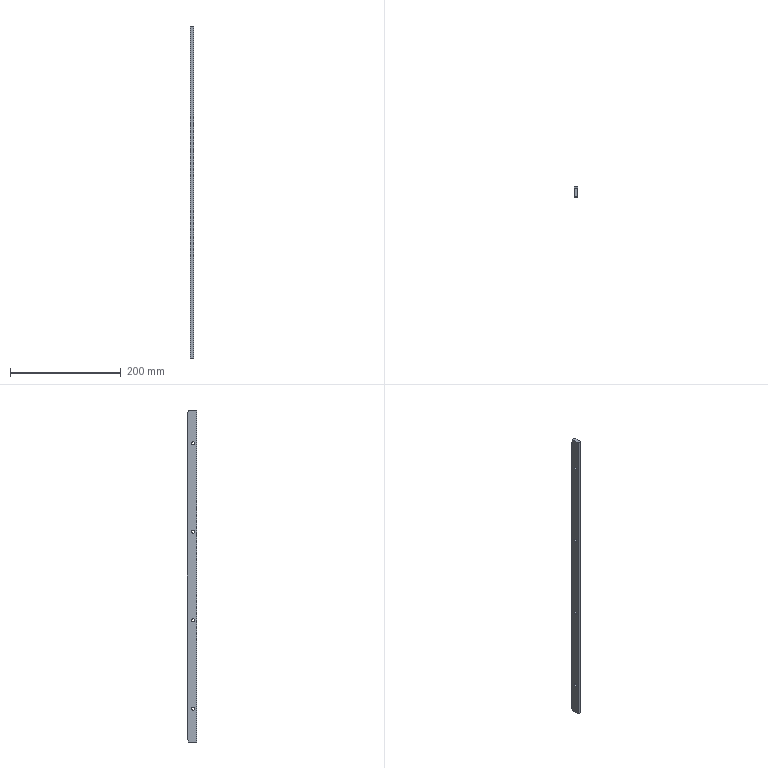Part | STEP file | 0228_206_Guide | 1 solid | 16 faces | box 6 x 18 x 600 mm | volume 64069 mm3 | cylinder 8 | plane 8 | commonest cylinder face diameters 5.5 x8
STEP:
#1=CARTESIAN_POINT('',(0.,0.,0.));
#2=DIRECTION('',(0.,0.,1.));
#3=DIRECTION('',(1.,0.,0.));
#4=AXIS2_PLACEMENT_3D('',#1,#2,#3);
#5=CARTESIAN_POINT('',(-6.,7.,237.25));
#6=VERTEX_POINT('',#5);
#7=CARTESIAN_POINT('',(0.,7.,237.25));
#8=VERTEX_POINT('',#7);
#9=CARTESIAN_POINT('',(0.,7.,237.25));
#10=DIRECTION('',(1.,0.,0.));
#11=VECTOR('',#10,1.);
#12=LINE('',#9,#11);
#13=CARTESIAN_POINT('',(0.,7.,240.));
#14=DIRECTION('',(1.,0.,0.));
#15=DIRECTION('',(0.,0.,-1.));
#16=AXIS2_PLACEMENT_3D('',#13,#14,#15);
#17=CYLINDRICAL_SURFACE('',#16,2.75);
#18=CARTESIAN_POINT('',(6.283,0.));
#19=DIRECTION('',(0.,1.));
#20=VECTOR('',#19,1.);
#21=LINE('',#18,#20);
#22=(GEOMETRIC_REPRESENTATION_CONTEXT(2)PARAMETRIC_REPRESENTATION_CONTEXT()REPRESENTATION_CONTEXT('',''));
#23=DEFINITIONAL_REPRESENTATION('',(#21),#22);
#24=PCURVE('',#17,#23);
#25=CARTESIAN_POINT('',(0.,7.,240.));
#26=DIRECTION('',(1.,0.,0.));
#27=DIRECTION('',(0.,0.,-1.));
#28=AXIS2_PLACEMENT_3D('',#25,#26,#27);
#29=CYLINDRICAL_SURFACE('',#28,2.75);
#30=CARTESIAN_POINT('',(0.,0.));
#31=DIRECTION('',(0.,1.));
#32=VECTOR('',#31,1.);
#33=LINE('',#30,#32);
#34=(GEOMETRIC_REPRESENTATION_CONTEXT(2)PARAMETRIC_REPRESENTATION_CONTEXT()REPRESENTATION_CONTEXT('',''));
#35=DEFINITIONAL_REPRESENTATION('',(#33),#34);
#36=PCURVE('',#29,#35);
#37=SURFACE_CURVE('',#12,(#24,#36),.PCURVE_S1.);
#38=EDGE_CURVE('',#6,#8,#37,.T.);
#39=ORIENTED_EDGE('',*,*,#38,.T.);
#40=CARTESIAN_POINT('',(0.,7.,242.75));
#41=VERTEX_POINT('',#40);
#42=CARTESIAN_POINT('',(0.,7.,240.));
#43=DIRECTION('',(1.,0.,0.));
#44=DIRECTION('',(0.,0.,-1.));
#45=AXIS2_PLACEMENT_3D('',#42,#43,#44);
#46=CIRCLE('',#45,2.75);
#47=CARTESIAN_POINT('',(0.,0.));
#48=DIRECTION('',(1.,0.));
#49=VECTOR('',#48,1.);
#50=LINE('',#47,#49);
#51=(GEOMETRIC_REPRESENTATION_CONTEXT(2)PARAMETRIC_REPRESENTATION_CONTEXT()REPRESENTATION_CONTEXT('',''));
#52=DEFINITIONAL_REPRESENTATION('',(#50),#51);
#53=PCURVE('',#17,#52);
#54=CARTESIAN_POINT('',(0.,18.,-300.));
#55=DIRECTION('',(1.,0.,0.));
#56=DIRECTION('',(0.,0.,-1.));
#57=AXIS2_PLACEMENT_3D('',#54,#55,#56);
#58=PLANE('',#57);
#59=CARTESIAN_POINT('',(-540.,-11.));
#60=DIRECTION('',(1.,0.));
#61=AXIS2_PLACEMENT_2D('',#59,#60);
#62=CIRCLE('',#61,2.75);
#63=(GEOMETRIC_REPRESENTATION_CONTEXT(2)PARAMETRIC_REPRESENTATION_CONTEXT()REPRESENTATION_CONTEXT('',''));
#64=DEFINITIONAL_REPRESENTATION('',(#62),#63);
#65=PCURVE('',#58,#64);
#66=SURFACE_CURVE('',#46,(#53,#65),.PCURVE_S1.);
#67=EDGE_CURVE('',#41,#8,#66,.T.);
#68=ORIENTED_EDGE('',*,*,#67,.F.);
#69=CARTESIAN_POINT('',(-6.,7.,242.75));
#70=VERTEX_POINT('',#69);
#71=CARTESIAN_POINT('',(0.,7.,242.75));
#72=DIRECTION('',(1.,0.,0.));
#73=VECTOR('',#72,1.);
#74=LINE('',#71,#73);
#75=CARTESIAN_POINT('',(3.142,0.));
#76=DIRECTION('',(0.,1.));
#77=VECTOR('',#76,1.);
#78=LINE('',#75,#77);
#79=(GEOMETRIC_REPRESENTATION_CONTEXT(2)PARAMETRIC_REPRESENTATION_CONTEXT()REPRESENTATION_CONTEXT('',''));
#80=DEFINITIONAL_REPRESENTATION('',(#78),#79);
#81=PCURVE('',#17,#80);
#82=CARTESIAN_POINT('',(3.142,0.));
#83=DIRECTION('',(0.,1.));
#84=VECTOR('',#83,1.);
#85=LINE('',#82,#84);
#86=(GEOMETRIC_REPRESENTATION_CONTEXT(2)PARAMETRIC_REPRESENTATION_CONTEXT()REPRESENTATION_CONTEXT('',''));
#87=DEFINITIONAL_REPRESENTATION('',(#85),#86);
#88=PCURVE('',#29,#87);
#89=SURFACE_CURVE('',#74,(#81,#88),.PCURVE_S1.);
#90=EDGE_CURVE('',#70,#41,#89,.T.);
#91=ORIENTED_EDGE('',*,*,#90,.F.);
#92=CARTESIAN_POINT('',(-6.,7.,240.));
#93=DIRECTION('',(1.,0.,0.));
#94=DIRECTION('',(0.,0.,-1.));
#95=AXIS2_PLACEMENT_3D('',#92,#93,#94);
#96=CIRCLE('',#95,2.75);
#97=CARTESIAN_POINT('',(0.,-6.));
#98=DIRECTION('',(1.,0.));
#99=VECTOR('',#98,1.);
#100=LINE('',#97,#99);
#101=(GEOMETRIC_REPRESENTATION_CONTEXT(2)PARAMETRIC_REPRESENTATION_CONTEXT()REPRESENTATION_CONTEXT('',''));
#102=DEFINITIONAL_REPRESENTATION('',(#100),#101);
#103=PCURVE('',#17,#102);
#104=CARTESIAN_POINT('',(-6.,18.,-300.));
#105=DIRECTION('',(1.,0.,0.));
#106=DIRECTION('',(0.,0.,-1.));
#107=AXIS2_PLACEMENT_3D('',#104,#105,#106);
#108=PLANE('',#107);
#109=CARTESIAN_POINT('',(-540.,-11.));
#110=DIRECTION('',(1.,0.));
#111=AXIS2_PLACEMENT_2D('',#109,#110);
#112=CIRCLE('',#111,2.75);
#113=(GEOMETRIC_REPRESENTATION_CONTEXT(2)PARAMETRIC_REPRESENTATION_CONTEXT()REPRESENTATION_CONTEXT('',''));
#114=DEFINITIONAL_REPRESENTATION('',(#112),#113);
#115=PCURVE('',#108,#114);
#116=SURFACE_CURVE('',#96,(#103,#115),.PCURVE_S1.);
#117=EDGE_CURVE('',#70,#6,#116,.T.);
#118=ORIENTED_EDGE('',*,*,#117,.T.);
#119=EDGE_LOOP('',(#39,#68,#91,#118));
#120=FACE_BOUND('',#119,.F.);
#121=ADVANCED_FACE('',(#120),#17,.F.);
#122=CARTESIAN_POINT('',(-6.,7.,77.25));
#123=VERTEX_POINT('',#122);
#124=CARTESIAN_POINT('',(0.,7.,77.25));
#125=VERTEX_POINT('',#124);
#126=CARTESIAN_POINT('',(0.,7.,77.25));
#127=DIRECTION('',(1.,0.,0.));
#128=VECTOR('',#127,1.);
#129=LINE('',#126,#128);
#130=CARTESIAN_POINT('',(0.,7.,80.));
#131=DIRECTION('',(1.,0.,0.));
#132=DIRECTION('',(0.,0.,-1.));
#133=AXIS2_PLACEMENT_3D('',#130,#131,#132);
#134=CYLINDRICAL_SURFACE('',#133,2.75);
#135=CARTESIAN_POINT('',(6.283,0.));
#136=DIRECTION('',(0.,1.));
#137=VECTOR('',#136,1.);
#138=LINE('',#135,#137);
#139=(GEOMETRIC_REPRESENTATION_CONTEXT(2)PARAMETRIC_REPRESENTATION_CONTEXT()REPRESENTATION_CONTEXT('',''));
#140=DEFINITIONAL_REPRESENTATION('',(#138),#139);
#141=PCURVE('',#134,#140);
#142=CARTESIAN_POINT('',(0.,7.,80.));
#143=DIRECTION('',(1.,0.,0.));
#144=DIRECTION('',(0.,0.,-1.));
#145=AXIS2_PLACEMENT_3D('',#142,#143,#144);
#146=CYLINDRICAL_SURFACE('',#145,2.75);
#147=CARTESIAN_POINT('',(0.,0.));
#148=DIRECTION('',(0.,1.));
#149=VECTOR('',#148,1.);
#150=LINE('',#147,#149);
#151=(GEOMETRIC_REPRESENTATION_CONTEXT(2)PARAMETRIC_REPRESENTATION_CONTEXT()REPRESENTATION_CONTEXT('',''));
#152=DEFINITIONAL_REPRESENTATION('',(#150),#151);
#153=PCURVE('',#146,#152);
#154=SURFACE_CURVE('',#129,(#141,#153),.PCURVE_S1.);
#155=EDGE_CURVE('',#123,#125,#154,.T.);
#156=ORIENTED_EDGE('',*,*,#155,.T.);
#157=CARTESIAN_POINT('',(0.,7.,82.75));
#158=VERTEX_POINT('',#157);
#159=CARTESIAN_POINT('',(0.,7.,80.));
#160=DIRECTION('',(1.,0.,0.));
#161=DIRECTION('',(0.,0.,-1.));
#162=AXIS2_PLACEMENT_3D('',#159,#160,#161);
#163=CIRCLE('',#162,2.75);
#164=CARTESIAN_POINT('',(0.,0.));
#165=DIRECTION('',(1.,0.));
#166=VECTOR('',#165,1.);
#167=LINE('',#164,#166);
#168=(GEOMETRIC_REPRESENTATION_CONTEXT(2)PARAMETRIC_REPRESENTATION_CONTEXT()REPRESENTATION_CONTEXT('',''));
#169=DEFINITIONAL_REPRESENTATION('',(#167),#168);
#170=PCURVE('',#134,#169);
#171=CARTESIAN_POINT('',(-380.,-11.));
#172=DIRECTION('',(1.,0.));
#173=AXIS2_PLACEMENT_2D('',#171,#172);
#174=CIRCLE('',#173,2.75);
#175=(GEOMETRIC_REPRESENTATION_CONTEXT(2)PARAMETRIC_REPRESENTATION_CONTEXT()REPRESENTATION_CONTEXT('',''));
#176=DEFINITIONAL_REPRESENTATION('',(#174),#175);
#177=PCURVE('',#58,#176);
#178=SURFACE_CURVE('',#163,(#170,#177),.PCURVE_S1.);
#179=EDGE_CURVE('',#158,#125,#178,.T.);
#180=ORIENTED_EDGE('',*,*,#179,.F.);
#181=CARTESIAN_POINT('',(-6.,7.,82.75));
#182=VERTEX_POINT('',#181);
#183=CARTESIAN_POINT('',(0.,7.,82.75));
#184=DIRECTION('',(1.,0.,0.));
#185=VECTOR('',#184,1.);
#186=LINE('',#183,#185);
#187=CARTESIAN_POINT('',(3.142,0.));
#188=DIRECTION('',(0.,1.));
#189=VECTOR('',#188,1.);
#190=LINE('',#187,#189);
#191=(GEOMETRIC_REPRESENTATION_CONTEXT(2)PARAMETRIC_REPRESENTATION_CONTEXT()REPRESENTATION_CONTEXT('',''));
#192=DEFINITIONAL_REPRESENTATION('',(#190),#191);
#193=PCURVE('',#134,#192);
#194=CARTESIAN_POINT('',(3.142,0.));
#195=DIRECTION('',(0.,1.));
#196=VECTOR('',#195,1.);
#197=LINE('',#194,#196);
#198=(GEOMETRIC_REPRESENTATION_CONTEXT(2)PARAMETRIC_REPRESENTATION_CONTEXT()REPRESENTATION_CONTEXT('',''));
#199=DEFINITIONAL_REPRESENTATION('',(#197),#198);
#200=PCURVE('',#146,#199);
#201=SURFACE_CURVE('',#186,(#193,#200),.PCURVE_S1.);
#202=EDGE_CURVE('',#182,#158,#201,.T.);
#203=ORIENTED_EDGE('',*,*,#202,.F.);
#204=CARTESIAN_POINT('',(-6.,7.,80.));
#205=DIRECTION('',(1.,0.,0.));
#206=DIRECTION('',(0.,0.,-1.));
#207=AXIS2_PLACEMENT_3D('',#204,#205,#206);
#208=CIRCLE('',#207,2.75);
#209=CARTESIAN_POINT('',(0.,-6.));
#210=DIRECTION('',(1.,0.));
#211=VECTOR('',#210,1.);
#212=LINE('',#209,#211);
#213=(GEOMETRIC_REPRESENTATION_CONTEXT(2)PARAMETRIC_REPRESENTATION_CONTEXT()REPRESENTATION_CONTEXT('',''));
#214=DEFINITIONAL_REPRESENTATION('',(#212),#213);
#215=PCURVE('',#134,#214);
#216=CARTESIAN_POINT('',(-380.,-11.));
#217=DIRECTION('',(1.,0.));
#218=AXIS2_PLACEMENT_2D('',#216,#217);
#219=CIRCLE('',#218,2.75);
#220=(GEOMETRIC_REPRESENTATION_CONTEXT(2)PARAMETRIC_REPRESENTATION_CONTEXT()REPRESENTATION_CONTEXT('',''));
#221=DEFINITIONAL_REPRESENTATION('',(#219),#220);
#222=PCURVE('',#108,#221);
#223=SURFACE_CURVE('',#208,(#215,#222),.PCURVE_S1.);
#224=EDGE_CURVE('',#182,#123,#223,.T.);
#225=ORIENTED_EDGE('',*,*,#224,.T.);
#226=EDGE_LOOP('',(#156,#180,#203,#225));
#227=FACE_BOUND('',#226,.F.);
#228=ADVANCED_FACE('',(#227),#134,.F.);
#229=CARTESIAN_POINT('',(-6.,7.,-82.75));
#230=VERTEX_POINT('',#229);
#231=CARTESIAN_POINT('',(0.,7.,-82.75));
#232=VERTEX_POINT('',#231);
#233=CARTESIAN_POINT('',(0.,7.,-82.75));
#234=DIRECTION('',(1.,0.,0.));
#235=VECTOR('',#234,1.);
#236=LINE('',#233,#235);
#237=CARTESIAN_POINT('',(0.,7.,-80.));
#238=DIRECTION('',(1.,0.,0.));
#239=DIRECTION('',(0.,0.,-1.));
#240=AXIS2_PLACEMENT_3D('',#237,#238,#239);
#241=CYLINDRICAL_SURFACE('',#240,2.75);
#242=CARTESIAN_POINT('',(6.283,0.));
#243=DIRECTION('',(0.,1.));
#244=VECTOR('',#243,1.);
#245=LINE('',#242,#244);
#246=(GEOMETRIC_REPRESENTATION_CONTEXT(2)PARAMETRIC_REPRESENTATION_CONTEXT()REPRESENTATION_CONTEXT('',''));
#247=DEFINITIONAL_REPRESENTATION('',(#245),#246);
#248=PCURVE('',#241,#247);
#249=CARTESIAN_POINT('',(0.,7.,-80.));
#250=DIRECTION('',(1.,0.,0.));
#251=DIRECTION('',(0.,0.,-1.));
#252=AXIS2_PLACEMENT_3D('',#249,#250,#251);
#253=CYLINDRICAL_SURFACE('',#252,2.75);
#254=CARTESIAN_POINT('',(0.,0.));
#255=DIRECTION('',(0.,1.));
#256=VECTOR('',#255,1.);
#257=LINE('',#254,#256);
#258=(GEOMETRIC_REPRESENTATION_CONTEXT(2)PARAMETRIC_REPRESENTATION_CONTEXT()REPRESENTATION_CONTEXT('',''));
#259=DEFINITIONAL_REPRESENTATION('',(#257),#258);
#260=PCURVE('',#253,#259);
#261=SURFACE_CURVE('',#236,(#248,#260),.PCURVE_S1.);
#262=EDGE_CURVE('',#230,#232,#261,.T.);
#263=ORIENTED_EDGE('',*,*,#262,.T.);
#264=CARTESIAN_POINT('',(0.,7.,-77.25));
#265=VERTEX_POINT('',#264);
#266=CARTESIAN_POINT('',(0.,7.,-80.));
#267=DIRECTION('',(1.,0.,0.));
#268=DIRECTION('',(0.,0.,-1.));
#269=AXIS2_PLACEMENT_3D('',#266,#267,#268);
#270=CIRCLE('',#269,2.75);
#271=CARTESIAN_POINT('',(0.,0.));
#272=DIRECTION('',(1.,0.));
#273=VECTOR('',#272,1.);
#274=LINE('',#271,#273);
#275=(GEOMETRIC_REPRESENTATION_CONTEXT(2)PARAMETRIC_REPRESENTATION_CONTEXT()REPRESENTATION_CONTEXT('',''));
#276=DEFINITIONAL_REPRESENTATION('',(#274),#275);
#277=PCURVE('',#241,#276);
#278=CARTESIAN_POINT('',(-220.,-11.));
#279=DIRECTION('',(1.,0.));
#280=AXIS2_PLACEMENT_2D('',#278,#279);
#281=CIRCLE('',#280,2.75);
#282=(GEOMETRIC_REPRESENTATION_CONTEXT(2)PARAMETRIC_REPRESENTATION_CONTEXT()REPRESENTATION_CONTEXT('',''));
#283=DEFINITIONAL_REPRESENTATION('',(#281),#282);
#284=PCURVE('',#58,#283);
#285=SURFACE_CURVE('',#270,(#277,#284),.PCURVE_S1.);
#286=EDGE_CURVE('',#265,#232,#285,.T.);
#287=ORIENTED_EDGE('',*,*,#286,.F.);
#288=CARTESIAN_POINT('',(-6.,7.,-77.25));
#289=VERTEX_POINT('',#288);
#290=CARTESIAN_POINT('',(0.,7.,-77.25));
#291=DIRECTION('',(1.,0.,0.));
#292=VECTOR('',#291,1.);
#293=LINE('',#290,#292);
#294=CARTESIAN_POINT('',(3.142,0.));
#295=DIRECTION('',(0.,1.));
#296=VECTOR('',#295,1.);
#297=LINE('',#294,#296);
#298=(GEOMETRIC_REPRESENTATION_CONTEXT(2)PARAMETRIC_REPRESENTATION_CONTEXT()REPRESENTATION_CONTEXT('',''));
#299=DEFINITIONAL_REPRESENTATION('',(#297),#298);
#300=PCURVE('',#241,#299);
#301=CARTESIAN_POINT('',(3.142,0.));
#302=DIRECTION('',(0.,1.));
#303=VECTOR('',#302,1.);
#304=LINE('',#301,#303);
#305=(GEOMETRIC_REPRESENTATION_CONTEXT(2)PARAMETRIC_REPRESENTATION_CONTEXT()REPRESENTATION_CONTEXT('',''));
#306=DEFINITIONAL_REPRESENTATION('',(#304),#305);
#307=PCURVE('',#253,#306);
#308=SURFACE_CURVE('',#293,(#300,#307),.PCURVE_S1.);
#309=EDGE_CURVE('',#289,#265,#308,.T.);
#310=ORIENTED_EDGE('',*,*,#309,.F.);
#311=CARTESIAN_POINT('',(-6.,7.,-80.));
#312=DIRECTION('',(1.,0.,0.));
#313=DIRECTION('',(0.,0.,-1.));
#314=AXIS2_PLACEMENT_3D('',#311,#312,#313);
#315=CIRCLE('',#314,2.75);
#316=CARTESIAN_POINT('',(0.,-6.));
#317=DIRECTION('',(1.,0.));
#318=VECTOR('',#317,1.);
#319=LINE('',#316,#318);
#320=(GEOMETRIC_REPRESENTATION_CONTEXT(2)PARAMETRIC_REPRESENTATION_CONTEXT()REPRESENTATION_CONTEXT('',''));
#321=DEFINITIONAL_REPRESENTATION('',(#319),#320);
#322=PCURVE('',#241,#321);
#323=CARTESIAN_POINT('',(-220.,-11.));
#324=DIRECTION('',(1.,0.));
#325=AXIS2_PLACEMENT_2D('',#323,#324);
#326=CIRCLE('',#325,2.75);
#327=(GEOMETRIC_REPRESENTATION_CONTEXT(2)PARAMETRIC_REPRESENTATION_CONTEXT()REPRESENTATION_CONTEXT('',''));
#328=DEFINITIONAL_REPRESENTATION('',(#326),#327);
#329=PCURVE('',#108,#328);
#330=SURFACE_CURVE('',#315,(#322,#329),.PCURVE_S1.);
#331=EDGE_CURVE('',#289,#230,#330,.T.);
#332=ORIENTED_EDGE('',*,*,#331,.T.);
#333=EDGE_LOOP('',(#263,#287,#310,#332));
#334=FACE_BOUND('',#333,.F.);
#335=ADVANCED_FACE('',(#334),#241,.F.);
#336=CARTESIAN_POINT('',(-6.,7.,-242.75));
#337=VERTEX_POINT('',#336);
#338=CARTESIAN_POINT('',(0.,7.,-242.75));
#339=VERTEX_POINT('',#338);
#340=CARTESIAN_POINT('',(0.,7.,-242.75));
#341=DIRECTION('',(1.,0.,0.));
#342=VECTOR('',#341,1.);
#343=LINE('',#340,#342);
#344=CARTESIAN_POINT('',(0.,7.,-240.));
#345=DIRECTION('',(1.,0.,0.));
#346=DIRECTION('',(0.,0.,-1.));
#347=AXIS2_PLACEMENT_3D('',#344,#345,#346);
#348=CYLINDRICAL_SURFACE('',#347,2.75);
#349=CARTESIAN_POINT('',(6.283,0.));
#350=DIRECTION('',(0.,1.));
#351=VECTOR('',#350,1.);
#352=LINE('',#349,#351);
#353=(GEOMETRIC_REPRESENTATION_CONTEXT(2)PARAMETRIC_REPRESENTATION_CONTEXT()REPRESENTATION_CONTEXT('',''));
#354=DEFINITIONAL_REPRESENTATION('',(#352),#353);
#355=PCURVE('',#348,#354);
#356=CARTESIAN_POINT('',(0.,7.,-240.));
#357=DIRECTION('',(1.,0.,0.));
#358=DIRECTION('',(0.,0.,-1.));
#359=AXIS2_PLACEMENT_3D('',#356,#357,#358);
#360=CYLINDRICAL_SURFACE('',#359,2.75);
#361=CARTESIAN_POINT('',(0.,0.));
#362=DIRECTION('',(0.,1.));
#363=VECTOR('',#362,1.);
#364=LINE('',#361,#363);
#365=(GEOMETRIC_REPRESENTATION_CONTEXT(2)PARAMETRIC_REPRESENTATION_CONTEXT()REPRESENTATION_CONTEXT('',''));
#366=DEFINITIONAL_REPRESENTATION('',(#364),#365);
#367=PCURVE('',#360,#366);
#368=SURFACE_CURVE('',#343,(#355,#367),.PCURVE_S1.);
#369=EDGE_CURVE('',#337,#339,#368,.T.);
#370=ORIENTED_EDGE('',*,*,#369,.T.);
#371=CARTESIAN_POINT('',(0.,7.,-237.25));
#372=VERTEX_POINT('',#371);
#373=CARTESIAN_POINT('',(0.,7.,-240.));
#374=DIRECTION('',(1.,0.,0.));
#375=DIRECTION('',(0.,0.,-1.));
#376=AXIS2_PLACEMENT_3D('',#373,#374,#375);
#377=CIRCLE('',#376,2.75);
#378=CARTESIAN_POINT('',(0.,0.));
#379=DIRECTION('',(1.,0.));
#380=VECTOR('',#379,1.);
#381=LINE('',#378,#380);
#382=(GEOMETRIC_REPRESENTATION_CONTEXT(2)PARAMETRIC_REPRESENTATION_CONTEXT()REPRESENTATION_CONTEXT('',''));
#383=DEFINITIONAL_REPRESENTATION('',(#381),#382);
#384=PCURVE('',#348,#383);
#385=CARTESIAN_POINT('',(-60.,-11.));
#386=DIRECTION('',(1.,0.));
#387=AXIS2_PLACEMENT_2D('',#385,#386);
#388=CIRCLE('',#387,2.75);
#389=(GEOMETRIC_REPRESENTATION_CONTEXT(2)PARAMETRIC_REPRESENTATION_CONTEXT()REPRESENTATION_CONTEXT('',''));
#390=DEFINITIONAL_REPRESENTATION('',(#388),#389);
#391=PCURVE('',#58,#390);
#392=SURFACE_CURVE('',#377,(#384,#391),.PCURVE_S1.);
#393=EDGE_CURVE('',#372,#339,#392,.T.);
#394=ORIENTED_EDGE('',*,*,#393,.F.);
#395=CARTESIAN_POINT('',(-6.,7.,-237.25));
#396=VERTEX_POINT('',#395);
#397=CARTESIAN_POINT('',(0.,7.,-237.25));
#398=DIRECTION('',(1.,0.,0.));
#399=VECTOR('',#398,1.);
#400=LINE('',#397,#399);
#401=CARTESIAN_POINT('',(3.142,0.));
#402=DIRECTION('',(0.,1.));
#403=VECTOR('',#402,1.);
#404=LINE('',#401,#403);
#405=(GEOMETRIC_REPRESENTATION_CONTEXT(2)PARAMETRIC_REPRESENTATION_CONTEXT()REPRESENTATION_CONTEXT('',''));
#406=DEFINITIONAL_REPRESENTATION('',(#404),#405);
#407=PCURVE('',#348,#406);
#408=CARTESIAN_POINT('',(3.142,0.));
#409=DIRECTION('',(0.,1.));
#410=VECTOR('',#409,1.);
#411=LINE('',#408,#410);
#412=(GEOMETRIC_REPRESENTATION_CONTEXT(2)PARAMETRIC_REPRESENTATION_CONTEXT()REPRESENTATION_CONTEXT('',''));
#413=DEFINITIONAL_REPRESENTATION('',(#411),#412);
#414=PCURVE('',#360,#413);
#415=SURFACE_CURVE('',#400,(#407,#414),.PCURVE_S1.);
#416=EDGE_CURVE('',#396,#372,#415,.T.);
#417=ORIENTED_EDGE('',*,*,#416,.F.);
#418=CARTESIAN_POINT('',(-6.,7.,-240.));
#419=DIRECTION('',(1.,0.,0.));
#420=DIRECTION('',(0.,0.,-1.));
#421=AXIS2_PLACEMENT_3D('',#418,#419,#420);
#422=CIRCLE('',#421,2.75);
#423=CARTESIAN_POINT('',(0.,-6.));
#424=DIRECTION('',(1.,0.));
#425=VECTOR('',#424,1.);
#426=LINE('',#423,#425);
#427=(GEOMETRIC_REPRESENTATION_CONTEXT(2)PARAMETRIC_REPRESENTATION_CONTEXT()REPRESENTATION_CONTEXT('',''));
#428=DEFINITIONAL_REPRESENTATION('',(#426),#427);
#429=PCURVE('',#348,#428);
#430=CARTESIAN_POINT('',(-60.,-11.));
#431=DIRECTION('',(1.,0.));
#432=AXIS2_PLACEMENT_2D('',#430,#431);
#433=CIRCLE('',#432,2.75);
#434=(GEOMETRIC_REPRESENTATION_CONTEXT(2)PARAMETRIC_REPRESENTATION_CONTEXT()REPRESENTATION_CONTEXT('',''));
#435=DEFINITIONAL_REPRESENTATION('',(#433),#434);
#436=PCURVE('',#108,#435);
#437=SURFACE_CURVE('',#422,(#429,#436),.PCURVE_S1.);
#438=EDGE_CURVE('',#396,#337,#437,.T.);
#439=ORIENTED_EDGE('',*,*,#438,.T.);
#440=EDGE_LOOP('',(#370,#394,#417,#439));
#441=FACE_BOUND('',#440,.F.);
#442=ADVANCED_FACE('',(#441),#348,.F.);
#443=CARTESIAN_POINT('',(-6.,0.,-300.));
#444=VERTEX_POINT('',#443);
#445=CARTESIAN_POINT('',(-6.,15.321,-300.));
#446=VERTEX_POINT('',#445);
#447=CARTESIAN_POINT('',(-6.,0.,-300.));
#448=DIRECTION('',(0.,1.,0.));
#449=VECTOR('',#448,1.);
#450=LINE('',#447,#449);
#451=CARTESIAN_POINT('',(-6.,0.,-300.));
#452=DIRECTION('',(0.,0.,-1.));
#453=DIRECTION('',(-1.,0.,0.));
#454=AXIS2_PLACEMENT_3D('',#451,#452,#453);
#455=PLANE('',#454);
#456=CARTESIAN_POINT('',(0.,0.));
#457=DIRECTION('',(0.,1.));
#458=VECTOR('',#457,1.);
#459=LINE('',#456,#458);
#460=(GEOMETRIC_REPRESENTATION_CONTEXT(2)PARAMETRIC_REPRESENTATION_CONTEXT()REPRESENTATION_CONTEXT('',''));
#461=DEFINITIONAL_REPRESENTATION('',(#459),#460);
#462=PCURVE('',#455,#461);
#463=CARTESIAN_POINT('',(0.,-18.));
#464=DIRECTION('',(0.,1.));
#465=VECTOR('',#464,1.);
#466=LINE('',#463,#465);
#467=(GEOMETRIC_REPRESENTATION_CONTEXT(2)PARAMETRIC_REPRESENTATION_CONTEXT()REPRESENTATION_CONTEXT('',''));
#468=DEFINITIONAL_REPRESENTATION('',(#466),#467);
#469=PCURVE('',#108,#468);
#470=SURFACE_CURVE('',#450,(#462,#469),.PCURVE_S1.);
#471=EDGE_CURVE('',#444,#446,#470,.T.);
#472=ORIENTED_EDGE('',*,*,#471,.T.);
#473=CARTESIAN_POINT('',(0.,15.321,-300.));
#474=VERTEX_POINT('',#473);
#475=CARTESIAN_POINT('',(-6.,15.321,-300.));
#476=DIRECTION('',(1.,0.,0.));
#477=VECTOR('',#476,1.);
#478=LINE('',#475,#477);
#479=CARTESIAN_POINT('',(0.,15.321));
#480=DIRECTION('',(-1.,0.));
#481=VECTOR('',#480,1.);
#482=LINE('',#479,#481);
#483=(GEOMETRIC_REPRESENTATION_CONTEXT(2)PARAMETRIC_REPRESENTATION_CONTEXT()REPRESENTATION_CONTEXT('',''));
#484=DEFINITIONAL_REPRESENTATION('',(#482),#483);
#485=PCURVE('',#455,#484);
#486=CARTESIAN_POINT('',(-6.,15.321,-300.));
#487=DIRECTION('',(0.,-0.9659,0.2588));
#488=DIRECTION('',(0.,-0.2588,-0.9659));
#489=AXIS2_PLACEMENT_3D('',#486,#487,#488);
#490=PLANE('',#489);
#491=CARTESIAN_POINT('',(0.,0.));
#492=DIRECTION('',(0.,1.));
#493=VECTOR('',#492,1.);
#494=LINE('',#491,#493);
#495=(GEOMETRIC_REPRESENTATION_CONTEXT(2)PARAMETRIC_REPRESENTATION_CONTEXT()REPRESENTATION_CONTEXT('',''));
#496=DEFINITIONAL_REPRESENTATION('',(#494),#495);
#497=PCURVE('',#490,#496);
#498=SURFACE_CURVE('',#478,(#485,#497),.PCURVE_S1.);
#499=EDGE_CURVE('',#446,#474,#498,.T.);
#500=ORIENTED_EDGE('',*,*,#499,.T.);
#501=CARTESIAN_POINT('',(0.,0.,-300.));
#502=VERTEX_POINT('',#501);
#503=CARTESIAN_POINT('',(0.,0.,-300.));
#504=DIRECTION('',(0.,1.,0.));
#505=VECTOR('',#504,1.);
#506=LINE('',#503,#505);
#507=CARTESIAN_POINT('',(-6.,0.));
#508=DIRECTION('',(0.,1.));
#509=VECTOR('',#508,1.);
#510=LINE('',#507,#509);
#511=(GEOMETRIC_REPRESENTATION_CONTEXT(2)PARAMETRIC_REPRESENTATION_CONTEXT()REPRESENTATION_CONTEXT('',''));
#512=DEFINITIONAL_REPRESENTATION('',(#510),#511);
#513=PCURVE('',#455,#512);
#514=CARTESIAN_POINT('',(0.,-18.));
#515=DIRECTION('',(0.,1.));
#516=VECTOR('',#515,1.);
#517=LINE('',#514,#516);
#518=(GEOMETRIC_REPRESENTATION_CONTEXT(2)PARAMETRIC_REPRESENTATION_CONTEXT()REPRESENTATION_CONTEXT('',''));
#519=DEFINITIONAL_REPRESENTATION('',(#517),#518);
#520=PCURVE('',#58,#519);
#521=SURFACE_CURVE('',#506,(#513,#520),.PCURVE_S1.);
#522=EDGE_CURVE('',#502,#474,#521,.T.);
#523=ORIENTED_EDGE('',*,*,#522,.F.);
#524=CARTESIAN_POINT('',(-6.,0.,-300.));
#525=DIRECTION('',(1.,0.,0.));
#526=VECTOR('',#525,1.);
#527=LINE('',#524,#526);
#528=CARTESIAN_POINT('',(0.,0.));
#529=DIRECTION('',(-1.,0.));
#530=VECTOR('',#529,1.);
#531=LINE('',#528,#530);
#532=(GEOMETRIC_REPRESENTATION_CONTEXT(2)PARAMETRIC_REPRESENTATION_CONTEXT()REPRESENTATION_CONTEXT('',''));
#533=DEFINITIONAL_REPRESENTATION('',(#531),#532);
#534=PCURVE('',#455,#533);
#535=CARTESIAN_POINT('',(-6.,0.,-300.));
#536=DIRECTION('',(0.,-1.,0.));
#537=DIRECTION('',(0.,0.,-1.));
#538=AXIS2_PLACEMENT_3D('',#535,#536,#537);
#539=PLANE('',#538);
#540=CARTESIAN_POINT('',(0.,0.));
#541=DIRECTION('',(0.,1.));
#542=VECTOR('',#541,1.);
#543=LINE('',#540,#542);
#544=(GEOMETRIC_REPRESENTATION_CONTEXT(2)PARAMETRIC_REPRESENTATION_CONTEXT()REPRESENTATION_CONTEXT('',''));
#545=DEFINITIONAL_REPRESENTATION('',(#543),#544);
#546=PCURVE('',#539,#545);
#547=SURFACE_CURVE('',#527,(#534,#546),.PCURVE_S1.);
#548=EDGE_CURVE('',#444,#502,#547,.T.);
#549=ORIENTED_EDGE('',*,*,#548,.F.);
#550=EDGE_LOOP('',(#472,#500,#523,#549));
#551=FACE_BOUND('',#550,.T.);
#552=ADVANCED_FACE('',(#551),#455,.T.);
#553=CARTESIAN_POINT('',(0.,0.,300.));
#554=VERTEX_POINT('',#553);
#555=CARTESIAN_POINT('',(0.,0.,-300.));
#556=DIRECTION('',(0.,0.,-1.));
#557=VECTOR('',#556,1.);
#558=LINE('',#555,#557);
#559=CARTESIAN_POINT('',(0.,6.));
#560=DIRECTION('',(1.,0.));
#561=VECTOR('',#560,1.);
#562=LINE('',#559,#561);
#563=(GEOMETRIC_REPRESENTATION_CONTEXT(2)PARAMETRIC_REPRESENTATION_CONTEXT()REPRESENTATION_CONTEXT('',''));
#564=DEFINITIONAL_REPRESENTATION('',(#562),#563);
#565=PCURVE('',#539,#564);
#566=CARTESIAN_POINT('',(0.,-18.));
#567=DIRECTION('',(1.,0.));
#568=VECTOR('',#567,1.);
#569=LINE('',#566,#568);
#570=(GEOMETRIC_REPRESENTATION_CONTEXT(2)PARAMETRIC_REPRESENTATION_CONTEXT()REPRESENTATION_CONTEXT('',''));
#571=DEFINITIONAL_REPRESENTATION('',(#569),#570);
#572=PCURVE('',#58,#571);
#573=SURFACE_CURVE('',#558,(#565,#572),.PCURVE_S1.);
#574=EDGE_CURVE('',#554,#502,#573,.T.);
#575=ORIENTED_EDGE('',*,*,#574,.F.);
#576=CARTESIAN_POINT('',(-6.,0.,300.));
#577=VERTEX_POINT('',#576);
#578=CARTESIAN_POINT('',(-6.,0.,300.));
#579=DIRECTION('',(1.,0.,0.));
#580=VECTOR('',#579,1.);
#581=LINE('',#578,#580);
#582=CARTESIAN_POINT('',(-600.,0.));
#583=DIRECTION('',(0.,1.));
#584=VECTOR('',#583,1.);
#585=LINE('',#582,#584);
#586=(GEOMETRIC_REPRESENTATION_CONTEXT(2)PARAMETRIC_REPRESENTATION_CONTEXT()REPRESENTATION_CONTEXT('',''));
#587=DEFINITIONAL_REPRESENTATION('',(#585),#586);
#588=PCURVE('',#539,#587);
#589=CARTESIAN_POINT('',(-6.,0.,300.));
#590=DIRECTION('',(0.,0.,1.));
#591=DIRECTION('',(1.,0.,0.));
#592=AXIS2_PLACEMENT_3D('',#589,#590,#591);
#593=PLANE('',#592);
#594=CARTESIAN_POINT('',(0.,0.));
#595=DIRECTION('',(1.,0.));
#596=VECTOR('',#595,1.);
#597=LINE('',#594,#596);
#598=(GEOMETRIC_REPRESENTATION_CONTEXT(2)PARAMETRIC_REPRESENTATION_CONTEXT()REPRESENTATION_CONTEXT('',''));
#599=DEFINITIONAL_REPRESENTATION('',(#597),#598);
#600=PCURVE('',#593,#599);
#601=SURFACE_CURVE('',#581,(#588,#600),.PCURVE_S1.);
#602=EDGE_CURVE('',#577,#554,#601,.T.);
#603=ORIENTED_EDGE('',*,*,#602,.F.);
#604=CARTESIAN_POINT('',(-6.,0.,-300.));
#605=DIRECTION('',(0.,0.,-1.));
#606=VECTOR('',#605,1.);
#607=LINE('',#604,#606);
#608=CARTESIAN_POINT('',(0.,0.));
#609=DIRECTION('',(1.,0.));
#610=VECTOR('',#609,1.);
#611=LINE('',#608,#610);
#612=(GEOMETRIC_REPRESENTATION_CONTEXT(2)PARAMETRIC_REPRESENTATION_CONTEXT()REPRESENTATION_CONTEXT('',''));
#613=DEFINITIONAL_REPRESENTATION('',(#611),#612);
#614=PCURVE('',#539,#613);
#615=CARTESIAN_POINT('',(0.,-18.));
#616=DIRECTION('',(1.,0.));
#617=VECTOR('',#616,1.);
#618=LINE('',#615,#617);
#619=(GEOMETRIC_REPRESENTATION_CONTEXT(2)PARAMETRIC_REPRESENTATION_CONTEXT()REPRESENTATION_CONTEXT('',''));
#620=DEFINITIONAL_REPRESENTATION('',(#618),#619);
#621=PCURVE('',#108,#620);
#622=SURFACE_CURVE('',#607,(#614,#621),.PCURVE_S1.);
#623=EDGE_CURVE('',#577,#444,#622,.T.);
#624=ORIENTED_EDGE('',*,*,#623,.T.);
#625=ORIENTED_EDGE('',*,*,#548,.T.);
#626=EDGE_LOOP('',(#575,#603,#624,#625));
#627=FACE_BOUND('',#626,.T.);
#628=ADVANCED_FACE('',(#627),#539,.T.);
#629=CARTESIAN_POINT('',(0.,15.321,300.));
#630=VERTEX_POINT('',#629);
#631=CARTESIAN_POINT('',(0.,0.,300.));
#632=DIRECTION('',(0.,-1.,0.));
#633=VECTOR('',#632,1.);
#634=LINE('',#631,#633);
#635=CARTESIAN_POINT('',(6.,0.));
#636=DIRECTION('',(0.,-1.));
#637=VECTOR('',#636,1.);
#638=LINE('',#635,#637);
#639=(GEOMETRIC_REPRESENTATION_CONTEXT(2)PARAMETRIC_REPRESENTATION_CONTEXT()REPRESENTATION_CONTEXT('',''));
#640=DEFINITIONAL_REPRESENTATION('',(#638),#639);
#641=PCURVE('',#593,#640);
#642=CARTESIAN_POINT('',(-600.,-18.));
#643=DIRECTION('',(0.,-1.));
#644=VECTOR('',#643,1.);
#645=LINE('',#642,#644);
#646=(GEOMETRIC_REPRESENTATION_CONTEXT(2)PARAMETRIC_REPRESENTATION_CONTEXT()REPRESENTATION_CONTEXT('',''));
#647=DEFINITIONAL_REPRESENTATION('',(#645),#646);
#648=PCURVE('',#58,#647);
#649=SURFACE_CURVE('',#634,(#641,#648),.PCURVE_S1.);
#650=EDGE_CURVE('',#630,#554,#649,.T.);
#651=ORIENTED_EDGE('',*,*,#650,.F.);
#652=CARTESIAN_POINT('',(-6.,15.321,300.));
#653=VERTEX_POINT('',#652);
#654=CARTESIAN_POINT('',(-6.,15.321,300.));
#655=DIRECTION('',(-1.,0.,0.));
#656=VECTOR('',#655,1.);
#657=LINE('',#654,#656);
#658=CARTESIAN_POINT('',(0.,15.321));
#659=DIRECTION('',(-1.,0.));
#660=VECTOR('',#659,1.);
#661=LINE('',#658,#660);
#662=(GEOMETRIC_REPRESENTATION_CONTEXT(2)PARAMETRIC_REPRESENTATION_CONTEXT()REPRESENTATION_CONTEXT('',''));
#663=DEFINITIONAL_REPRESENTATION('',(#661),#662);
#664=PCURVE('',#593,#663);
#665=CARTESIAN_POINT('',(-6.,18.,290.));
#666=DIRECTION('',(0.,-0.9659,-0.2588));
#667=DIRECTION('',(0.,0.2588,-0.9659));
#668=AXIS2_PLACEMENT_3D('',#665,#666,#667);
#669=PLANE('',#668);
#670=CARTESIAN_POINT('',(-10.353,0.));
#671=DIRECTION('',(0.,-1.));
#672=VECTOR('',#671,1.);
#673=LINE('',#670,#672);
#674=(GEOMETRIC_REPRESENTATION_CONTEXT(2)PARAMETRIC_REPRESENTATION_CONTEXT()REPRESENTATION_CONTEXT('',''));
#675=DEFINITIONAL_REPRESENTATION('',(#673),#674);
#676=PCURVE('',#669,#675);
#677=SURFACE_CURVE('',#657,(#664,#676),.PCURVE_S1.);
#678=EDGE_CURVE('',#630,#653,#677,.T.);
#679=ORIENTED_EDGE('',*,*,#678,.T.);
#680=CARTESIAN_POINT('',(-6.,0.,300.));
#681=DIRECTION('',(0.,-1.,0.));
#682=VECTOR('',#681,1.);
#683=LINE('',#680,#682);
#684=CARTESIAN_POINT('',(0.,0.));
#685=DIRECTION('',(0.,-1.));
#686=VECTOR('',#685,1.);
#687=LINE('',#684,#686);
#688=(GEOMETRIC_REPRESENTATION_CONTEXT(2)PARAMETRIC_REPRESENTATION_CONTEXT()REPRESENTATION_CONTEXT('',''));
#689=DEFINITIONAL_REPRESENTATION('',(#687),#688);
#690=PCURVE('',#593,#689);
#691=CARTESIAN_POINT('',(-600.,-18.));
#692=DIRECTION('',(0.,-1.));
#693=VECTOR('',#692,1.);
#694=LINE('',#691,#693);
#695=(GEOMETRIC_REPRESENTATION_CONTEXT(2)PARAMETRIC_REPRESENTATION_CONTEXT()REPRESENTATION_CONTEXT('',''));
#696=DEFINITIONAL_REPRESENTATION('',(#694),#695);
#697=PCURVE('',#108,#696);
#698=SURFACE_CURVE('',#683,(#690,#697),.PCURVE_S1.);
#699=EDGE_CURVE('',#653,#577,#698,.T.);
#700=ORIENTED_EDGE('',*,*,#699,.T.);
#701=ORIENTED_EDGE('',*,*,#602,.T.);
#702=EDGE_LOOP('',(#651,#679,#700,#701));
#703=FACE_BOUND('',#702,.T.);
#704=ADVANCED_FACE('',(#703),#593,.T.);
#705=CARTESIAN_POINT('',(0.,18.,-290.));
#706=VERTEX_POINT('',#705);
#707=CARTESIAN_POINT('',(0.,18.,290.));
#708=VERTEX_POINT('',#707);
#709=CARTESIAN_POINT('',(0.,18.,-300.));
#710=DIRECTION('',(0.,0.,1.));
#711=VECTOR('',#710,1.);
#712=LINE('',#709,#711);
#713=CARTESIAN_POINT('',(-6.,18.,-300.));
#714=DIRECTION('',(0.,1.,0.));
#715=DIRECTION('',(0.,0.,1.));
#716=AXIS2_PLACEMENT_3D('',#713,#714,#715);
#717=PLANE('',#716);
#718=CARTESIAN_POINT('',(0.,6.));
#719=DIRECTION('',(1.,0.));
#720=VECTOR('',#719,1.);
#721=LINE('',#718,#720);
#722=(GEOMETRIC_REPRESENTATION_CONTEXT(2)PARAMETRIC_REPRESENTATION_CONTEXT()REPRESENTATION_CONTEXT('',''));
#723=DEFINITIONAL_REPRESENTATION('',(#721),#722);
#724=PCURVE('',#717,#723);
#725=CARTESIAN_POINT('',(0.,0.));
#726=DIRECTION('',(-1.,0.));
#727=VECTOR('',#726,1.);
#728=LINE('',#725,#727);
#729=(GEOMETRIC_REPRESENTATION_CONTEXT(2)PARAMETRIC_REPRESENTATION_CONTEXT()REPRESENTATION_CONTEXT('',''));
#730=DEFINITIONAL_REPRESENTATION('',(#728),#729);
#731=PCURVE('',#58,#730);
#732=SURFACE_CURVE('',#712,(#724,#731),.PCURVE_S1.);
#733=EDGE_CURVE('',#706,#708,#732,.T.);
#734=ORIENTED_EDGE('',*,*,#733,.F.);
#735=CARTESIAN_POINT('',(-6.,18.,-290.));
#736=VERTEX_POINT('',#735);
#737=CARTESIAN_POINT('',(-6.,18.,-290.));
#738=DIRECTION('',(-1.,0.,0.));
#739=VECTOR('',#738,1.);
#740=LINE('',#737,#739);
#741=CARTESIAN_POINT('',(10.,0.));
#742=DIRECTION('',(0.,-1.));
#743=VECTOR('',#742,1.);
#744=LINE('',#741,#743);
#745=(GEOMETRIC_REPRESENTATION_CONTEXT(2)PARAMETRIC_REPRESENTATION_CONTEXT()REPRESENTATION_CONTEXT('',''));
#746=DEFINITIONAL_REPRESENTATION('',(#744),#745);
#747=PCURVE('',#717,#746);
#748=CARTESIAN_POINT('',(-10.353,0.));
#749=DIRECTION('',(0.,-1.));
#750=VECTOR('',#749,1.);
#751=LINE('',#748,#750);
#752=(GEOMETRIC_REPRESENTATION_CONTEXT(2)PARAMETRIC_REPRESENTATION_CONTEXT()REPRESENTATION_CONTEXT('',''));
#753=DEFINITIONAL_REPRESENTATION('',(#751),#752);
#754=PCURVE('',#490,#753);
#755=SURFACE_CURVE('',#740,(#747,#754),.PCURVE_S1.);
#756=EDGE_CURVE('',#706,#736,#755,.T.);
#757=ORIENTED_EDGE('',*,*,#756,.T.);
#758=CARTESIAN_POINT('',(-6.,18.,290.));
#759=VERTEX_POINT('',#758);
#760=CARTESIAN_POINT('',(-6.,18.,-300.));
#761=DIRECTION('',(0.,0.,1.));
#762=VECTOR('',#761,1.);
#763=LINE('',#760,#762);
#764=CARTESIAN_POINT('',(0.,0.));
#765=DIRECTION('',(1.,0.));
#766=VECTOR('',#765,1.);
#767=LINE('',#764,#766);
#768=(GEOMETRIC_REPRESENTATION_CONTEXT(2)PARAMETRIC_REPRESENTATION_CONTEXT()REPRESENTATION_CONTEXT('',''));
#769=DEFINITIONAL_REPRESENTATION('',(#767),#768);
#770=PCURVE('',#717,#769);
#771=CARTESIAN_POINT('',(0.,0.));
#772=DIRECTION('',(-1.,0.));
#773=VECTOR('',#772,1.);
#774=LINE('',#771,#773);
#775=(GEOMETRIC_REPRESENTATION_CONTEXT(2)PARAMETRIC_REPRESENTATION_CONTEXT()REPRESENTATION_CONTEXT('',''));
#776=DEFINITIONAL_REPRESENTATION('',(#774),#775);
#777=PCURVE('',#108,#776);
#778=SURFACE_CURVE('',#763,(#770,#777),.PCURVE_S1.);
#779=EDGE_CURVE('',#736,#759,#778,.T.);
#780=ORIENTED_EDGE('',*,*,#779,.T.);
#781=CARTESIAN_POINT('',(-6.,18.,290.));
#782=DIRECTION('',(1.,0.,0.));
#783=VECTOR('',#782,1.);
#784=LINE('',#781,#783);
#785=CARTESIAN_POINT('',(590.,0.));
#786=DIRECTION('',(0.,1.));
#787=VECTOR('',#786,1.);
#788=LINE('',#785,#787);
#789=(GEOMETRIC_REPRESENTATION_CONTEXT(2)PARAMETRIC_REPRESENTATION_CONTEXT()REPRESENTATION_CONTEXT('',''));
#790=DEFINITIONAL_REPRESENTATION('',(#788),#789);
#791=PCURVE('',#717,#790);
#792=CARTESIAN_POINT('',(0.,0.));
#793=DIRECTION('',(0.,1.));
#794=VECTOR('',#793,1.);
#795=LINE('',#792,#794);
#796=(GEOMETRIC_REPRESENTATION_CONTEXT(2)PARAMETRIC_REPRESENTATION_CONTEXT()REPRESENTATION_CONTEXT('',''));
#797=DEFINITIONAL_REPRESENTATION('',(#795),#796);
#798=PCURVE('',#669,#797);
#799=SURFACE_CURVE('',#784,(#791,#798),.PCURVE_S1.);
#800=EDGE_CURVE('',#759,#708,#799,.T.);
#801=ORIENTED_EDGE('',*,*,#800,.T.);
#802=EDGE_LOOP('',(#734,#757,#780,#801));
#803=FACE_BOUND('',#802,.T.);
#804=ADVANCED_FACE('',(#803),#717,.T.);
#805=CARTESIAN_POINT('',(-6.,7.,240.));
#806=DIRECTION('',(1.,0.,0.));
#807=DIRECTION('',(0.,0.,-1.));
#808=AXIS2_PLACEMENT_3D('',#805,#806,#807);
#809=CIRCLE('',#808,2.75);
#810=CARTESIAN_POINT('',(-540.,-11.));
#811=DIRECTION('',(1.,0.));
#812=AXIS2_PLACEMENT_2D('',#810,#811);
#813=CIRCLE('',#812,2.75);
#814=(GEOMETRIC_REPRESENTATION_CONTEXT(2)PARAMETRIC_REPRESENTATION_CONTEXT()REPRESENTATION_CONTEXT('',''));
#815=DEFINITIONAL_REPRESENTATION('',(#813),#814);
#816=PCURVE('',#108,#815);
#817=CARTESIAN_POINT('',(0.,-6.));
#818=DIRECTION('',(1.,0.));
#819=VECTOR('',#818,1.);
#820=LINE('',#817,#819);
#821=(GEOMETRIC_REPRESENTATION_CONTEXT(2)PARAMETRIC_REPRESENTATION_CONTEXT()REPRESENTATION_CONTEXT('',''));
#822=DEFINITIONAL_REPRESENTATION('',(#820),#821);
#823=PCURVE('',#29,#822);
#824=SURFACE_CURVE('',#809,(#816,#823),.PCURVE_S1.);
#825=EDGE_CURVE('',#6,#70,#824,.T.);
#826=ORIENTED_EDGE('',*,*,#825,.T.);
#827=ORIENTED_EDGE('',*,*,#117,.T.);
#828=EDGE_LOOP('',(#826,#827));
#829=FACE_BOUND('',#828,.T.);
#830=CARTESIAN_POINT('',(-6.,7.,80.));
#831=DIRECTION('',(1.,0.,0.));
#832=DIRECTION('',(0.,0.,-1.));
#833=AXIS2_PLACEMENT_3D('',#830,#831,#832);
#834=CIRCLE('',#833,2.75);
#835=CARTESIAN_POINT('',(-380.,-11.));
#836=DIRECTION('',(1.,0.));
#837=AXIS2_PLACEMENT_2D('',#835,#836);
#838=CIRCLE('',#837,2.75);
#839=(GEOMETRIC_REPRESENTATION_CONTEXT(2)PARAMETRIC_REPRESENTATION_CONTEXT()REPRESENTATION_CONTEXT('',''));
#840=DEFINITIONAL_REPRESENTATION('',(#838),#839);
#841=PCURVE('',#108,#840);
#842=CARTESIAN_POINT('',(0.,-6.));
#843=DIRECTION('',(1.,0.));
#844=VECTOR('',#843,1.);
#845=LINE('',#842,#844);
#846=(GEOMETRIC_REPRESENTATION_CONTEXT(2)PARAMETRIC_REPRESENTATION_CONTEXT()REPRESENTATION_CONTEXT('',''));
#847=DEFINITIONAL_REPRESENTATION('',(#845),#846);
#848=PCURVE('',#146,#847);
#849=SURFACE_CURVE('',#834,(#841,#848),.PCURVE_S1.);
#850=EDGE_CURVE('',#123,#182,#849,.T.);
#851=ORIENTED_EDGE('',*,*,#850,.T.);
#852=ORIENTED_EDGE('',*,*,#224,.T.);
#853=EDGE_LOOP('',(#851,#852));
#854=FACE_BOUND('',#853,.T.);
#855=CARTESIAN_POINT('',(-6.,7.,-80.));
#856=DIRECTION('',(1.,0.,0.));
#857=DIRECTION('',(0.,0.,-1.));
#858=AXIS2_PLACEMENT_3D('',#855,#856,#857);
#859=CIRCLE('',#858,2.75);
#860=CARTESIAN_POINT('',(-220.,-11.));
#861=DIRECTION('',(1.,0.));
#862=AXIS2_PLACEMENT_2D('',#860,#861);
#863=CIRCLE('',#862,2.75);
#864=(GEOMETRIC_REPRESENTATION_CONTEXT(2)PARAMETRIC_REPRESENTATION_CONTEXT()REPRESENTATION_CONTEXT('',''));
#865=DEFINITIONAL_REPRESENTATION('',(#863),#864);
#866=PCURVE('',#108,#865);
#867=CARTESIAN_POINT('',(0.,-6.));
#868=DIRECTION('',(1.,0.));
#869=VECTOR('',#868,1.);
#870=LINE('',#867,#869);
#871=(GEOMETRIC_REPRESENTATION_CONTEXT(2)PARAMETRIC_REPRESENTATION_CONTEXT()REPRESENTATION_CONTEXT('',''));
#872=DEFINITIONAL_REPRESENTATION('',(#870),#871);
#873=PCURVE('',#253,#872);
#874=SURFACE_CURVE('',#859,(#866,#873),.PCURVE_S1.);
#875=EDGE_CURVE('',#230,#289,#874,.T.);
#876=ORIENTED_EDGE('',*,*,#875,.T.);
#877=ORIENTED_EDGE('',*,*,#331,.T.);
#878=EDGE_LOOP('',(#876,#877));
#879=FACE_BOUND('',#878,.T.);
#880=CARTESIAN_POINT('',(-6.,7.,-240.));
#881=DIRECTION('',(1.,0.,0.));
#882=DIRECTION('',(0.,0.,-1.));
#883=AXIS2_PLACEMENT_3D('',#880,#881,#882);
#884=CIRCLE('',#883,2.75);
#885=CARTESIAN_POINT('',(-60.,-11.));
#886=DIRECTION('',(1.,0.));
#887=AXIS2_PLACEMENT_2D('',#885,#886);
#888=CIRCLE('',#887,2.75);
#889=(GEOMETRIC_REPRESENTATION_CONTEXT(2)PARAMETRIC_REPRESENTATION_CONTEXT()REPRESENTATION_CONTEXT('',''));
#890=DEFINITIONAL_REPRESENTATION('',(#888),#889);
#891=PCURVE('',#108,#890);
#892=CARTESIAN_POINT('',(0.,-6.));
#893=DIRECTION('',(1.,0.));
#894=VECTOR('',#893,1.);
#895=LINE('',#892,#894);
#896=(GEOMETRIC_REPRESENTATION_CONTEXT(2)PARAMETRIC_REPRESENTATION_CONTEXT()REPRESENTATION_CONTEXT('',''));
#897=DEFINITIONAL_REPRESENTATION('',(#895),#896);
#898=PCURVE('',#360,#897);
#899=SURFACE_CURVE('',#884,(#891,#898),.PCURVE_S1.);
#900=EDGE_CURVE('',#337,#396,#899,.T.);
#901=ORIENTED_EDGE('',*,*,#900,.T.);
#902=ORIENTED_EDGE('',*,*,#438,.T.);
#903=EDGE_LOOP('',(#901,#902));
#904=FACE_BOUND('',#903,.T.);
#905=ORIENTED_EDGE('',*,*,#779,.F.);
#906=CARTESIAN_POINT('',(-6.,15.321,-300.));
#907=DIRECTION('',(0.,-0.2588,-0.9659));
#908=VECTOR('',#907,1.);
#909=LINE('',#906,#908);
#910=CARTESIAN_POINT('',(0.,-2.679));
#911=DIRECTION('',(0.9659,-0.2588));
#912=VECTOR('',#911,1.);
#913=LINE('',#910,#912);
#914=(GEOMETRIC_REPRESENTATION_CONTEXT(2)PARAMETRIC_REPRESENTATION_CONTEXT()REPRESENTATION_CONTEXT('',''));
#915=DEFINITIONAL_REPRESENTATION('',(#913),#914);
#916=PCURVE('',#108,#915);
#917=CARTESIAN_POINT('',(0.,0.));
#918=DIRECTION('',(1.,0.));
#919=VECTOR('',#918,1.);
#920=LINE('',#917,#919);
#921=(GEOMETRIC_REPRESENTATION_CONTEXT(2)PARAMETRIC_REPRESENTATION_CONTEXT()REPRESENTATION_CONTEXT('',''));
#922=DEFINITIONAL_REPRESENTATION('',(#920),#921);
#923=PCURVE('',#490,#922);
#924=SURFACE_CURVE('',#909,(#916,#923),.PCURVE_S1.);
#925=EDGE_CURVE('',#736,#446,#924,.T.);
#926=ORIENTED_EDGE('',*,*,#925,.T.);
#927=ORIENTED_EDGE('',*,*,#471,.F.);
#928=ORIENTED_EDGE('',*,*,#623,.F.);
#929=ORIENTED_EDGE('',*,*,#699,.F.);
#930=CARTESIAN_POINT('',(-6.,18.,290.));
#931=DIRECTION('',(0.,0.2588,-0.9659));
#932=VECTOR('',#931,1.);
#933=LINE('',#930,#932);
#934=CARTESIAN_POINT('',(-590.,0.));
#935=DIRECTION('',(0.9659,0.2588));
#936=VECTOR('',#935,1.);
#937=LINE('',#934,#936);
#938=(GEOMETRIC_REPRESENTATION_CONTEXT(2)PARAMETRIC_REPRESENTATION_CONTEXT()REPRESENTATION_CONTEXT('',''));
#939=DEFINITIONAL_REPRESENTATION('',(#937),#938);
#940=PCURVE('',#108,#939);
#941=CARTESIAN_POINT('',(0.,0.));
#942=DIRECTION('',(1.,0.));
#943=VECTOR('',#942,1.);
#944=LINE('',#941,#943);
#945=(GEOMETRIC_REPRESENTATION_CONTEXT(2)PARAMETRIC_REPRESENTATION_CONTEXT()REPRESENTATION_CONTEXT('',''));
#946=DEFINITIONAL_REPRESENTATION('',(#944),#945);
#947=PCURVE('',#669,#946);
#948=SURFACE_CURVE('',#933,(#940,#947),.PCURVE_S1.);
#949=EDGE_CURVE('',#653,#759,#948,.T.);
#950=ORIENTED_EDGE('',*,*,#949,.T.);
#951=EDGE_LOOP('',(#905,#926,#927,#928,#929,#950));
#952=FACE_BOUND('',#951,.T.);
#953=ADVANCED_FACE('',(#829,#854,#879,#904,#952),#108,.F.);
#954=CARTESIAN_POINT('',(0.,7.,240.));
#955=DIRECTION('',(1.,0.,0.));
#956=DIRECTION('',(0.,0.,-1.));
#957=AXIS2_PLACEMENT_3D('',#954,#955,#956);
#958=CIRCLE('',#957,2.75);
#959=CARTESIAN_POINT('',(-540.,-11.));
#960=DIRECTION('',(1.,0.));
#961=AXIS2_PLACEMENT_2D('',#959,#960);
#962=CIRCLE('',#961,2.75);
#963=(GEOMETRIC_REPRESENTATION_CONTEXT(2)PARAMETRIC_REPRESENTATION_CONTEXT()REPRESENTATION_CONTEXT('',''));
#964=DEFINITIONAL_REPRESENTATION('',(#962),#963);
#965=PCURVE('',#58,#964);
#966=CARTESIAN_POINT('',(0.,0.));
#967=DIRECTION('',(1.,0.));
#968=VECTOR('',#967,1.);
#969=LINE('',#966,#968);
#970=(GEOMETRIC_REPRESENTATION_CONTEXT(2)PARAMETRIC_REPRESENTATION_CONTEXT()REPRESENTATION_CONTEXT('',''));
#971=DEFINITIONAL_REPRESENTATION('',(#969),#970);
#972=PCURVE('',#29,#971);
#973=SURFACE_CURVE('',#958,(#965,#972),.PCURVE_S1.);
#974=EDGE_CURVE('',#8,#41,#973,.T.);
#975=ORIENTED_EDGE('',*,*,#974,.F.);
#976=ORIENTED_EDGE('',*,*,#67,.F.);
#977=EDGE_LOOP('',(#975,#976));
#978=FACE_BOUND('',#977,.T.);
#979=CARTESIAN_POINT('',(0.,7.,80.));
#980=DIRECTION('',(1.,0.,0.));
#981=DIRECTION('',(0.,0.,-1.));
#982=AXIS2_PLACEMENT_3D('',#979,#980,#981);
#983=CIRCLE('',#982,2.75);
#984=CARTESIAN_POINT('',(-380.,-11.));
#985=DIRECTION('',(1.,0.));
#986=AXIS2_PLACEMENT_2D('',#984,#985);
#987=CIRCLE('',#986,2.75);
#988=(GEOMETRIC_REPRESENTATION_CONTEXT(2)PARAMETRIC_REPRESENTATION_CONTEXT()REPRESENTATION_CONTEXT('',''));
#989=DEFINITIONAL_REPRESENTATION('',(#987),#988);
#990=PCURVE('',#58,#989);
#991=CARTESIAN_POINT('',(0.,0.));
#992=DIRECTION('',(1.,0.));
#993=VECTOR('',#992,1.);
#994=LINE('',#991,#993);
#995=(GEOMETRIC_REPRESENTATION_CONTEXT(2)PARAMETRIC_REPRESENTATION_CONTEXT()REPRESENTATION_CONTEXT('',''));
#996=DEFINITIONAL_REPRESENTATION('',(#994),#995);
#997=PCURVE('',#146,#996);
#998=SURFACE_CURVE('',#983,(#990,#997),.PCURVE_S1.);
#999=EDGE_CURVE('',#125,#158,#998,.T.);
#1000=ORIENTED_EDGE('',*,*,#999,.F.);
#1001=ORIENTED_EDGE('',*,*,#179,.F.);
#1002=EDGE_LOOP('',(#1000,#1001));
#1003=FACE_BOUND('',#1002,.T.);
#1004=CARTESIAN_POINT('',(0.,7.,-80.));
#1005=DIRECTION('',(1.,0.,0.));
#1006=DIRECTION('',(0.,0.,-1.));
#1007=AXIS2_PLACEMENT_3D('',#1004,#1005,#1006);
#1008=CIRCLE('',#1007,2.75);
#1009=CARTESIAN_POINT('',(-220.,-11.));
#1010=DIRECTION('',(1.,0.));
#1011=AXIS2_PLACEMENT_2D('',#1009,#1010);
#1012=CIRCLE('',#1011,2.75);
#1013=(GEOMETRIC_REPRESENTATION_CONTEXT(2)PARAMETRIC_REPRESENTATION_CONTEXT()REPRESENTATION_CONTEXT('',''));
#1014=DEFINITIONAL_REPRESENTATION('',(#1012),#1013);
#1015=PCURVE('',#58,#1014);
#1016=CARTESIAN_POINT('',(0.,0.));
#1017=DIRECTION('',(1.,0.));
#1018=VECTOR('',#1017,1.);
#1019=LINE('',#1016,#1018);
#1020=(GEOMETRIC_REPRESENTATION_CONTEXT(2)PARAMETRIC_REPRESENTATION_CONTEXT()REPRESENTATION_CONTEXT('',''));
#1021=DEFINITIONAL_REPRESENTATION('',(#1019),#1020);
#1022=PCURVE('',#253,#1021);
#1023=SURFACE_CURVE('',#1008,(#1015,#1022),.PCURVE_S1.);
#1024=EDGE_CURVE('',#232,#265,#1023,.T.);
#1025=ORIENTED_EDGE('',*,*,#1024,.F.);
#1026=ORIENTED_EDGE('',*,*,#286,.F.);
#1027=EDGE_LOOP('',(#1025,#1026));
#1028=FACE_BOUND('',#1027,.T.);
#1029=CARTESIAN_POINT('',(0.,7.,-240.));
#1030=DIRECTION('',(1.,0.,0.));
#1031=DIRECTION('',(0.,0.,-1.));
#1032=AXIS2_PLACEMENT_3D('',#1029,#1030,#1031);
#1033=CIRCLE('',#1032,2.75);
#1034=CARTESIAN_POINT('',(-60.,-11.));
#1035=DIRECTION('',(1.,0.));
#1036=AXIS2_PLACEMENT_2D('',#1034,#1035);
#1037=CIRCLE('',#1036,2.75);
#1038=(GEOMETRIC_REPRESENTATION_CONTEXT(2)PARAMETRIC_REPRESENTATION_CONTEXT()REPRESENTATION_CONTEXT('',''));
#1039=DEFINITIONAL_REPRESENTATION('',(#1037),#1038);
#1040=PCURVE('',#58,#1039);
#1041=CARTESIAN_POINT('',(0.,0.));
#1042=DIRECTION('',(1.,0.));
#1043=VECTOR('',#1042,1.);
#1044=LINE('',#1041,#1043);
#1045=(GEOMETRIC_REPRESENTATION_CONTEXT(2)PARAMETRIC_REPRESENTATION_CONTEXT()REPRESENTATION_CONTEXT('',''));
#1046=DEFINITIONAL_REPRESENTATION('',(#1044),#1045);
#1047=PCURVE('',#360,#1046);
#1048=SURFACE_CURVE('',#1033,(#1040,#1047),.PCURVE_S1.);
#1049=EDGE_CURVE('',#339,#372,#1048,.T.);
#1050=ORIENTED_EDGE('',*,*,#1049,.F.);
#1051=ORIENTED_EDGE('',*,*,#393,.F.);
#1052=EDGE_LOOP('',(#1050,#1051));
#1053=FACE_BOUND('',#1052,.T.);
#1054=ORIENTED_EDGE('',*,*,#522,.T.);
#1055=CARTESIAN_POINT('',(0.,15.5,-299.33));
#1056=DIRECTION('',(0.,0.2588,0.9659));
#1057=VECTOR('',#1056,1.);
#1058=LINE('',#1055,#1057);
#1059=CARTESIAN_POINT('',(-0.6699,-2.5));
#1060=DIRECTION('',(-0.9659,0.2588));
#1061=VECTOR('',#1060,1.);
#1062=LINE('',#1059,#1061);
#1063=(GEOMETRIC_REPRESENTATION_CONTEXT(2)PARAMETRIC_REPRESENTATION_CONTEXT()REPRESENTATION_CONTEXT('',''));
#1064=DEFINITIONAL_REPRESENTATION('',(#1062),#1063);
#1065=PCURVE('',#58,#1064);
#1066=CARTESIAN_POINT('',(-0.6935,6.));
#1067=DIRECTION('',(-1.,0.));
#1068=VECTOR('',#1067,1.);
#1069=LINE('',#1066,#1068);
#1070=(GEOMETRIC_REPRESENTATION_CONTEXT(2)PARAMETRIC_REPRESENTATION_CONTEXT()REPRESENTATION_CONTEXT('',''));
#1071=DEFINITIONAL_REPRESENTATION('',(#1069),#1070);
#1072=PCURVE('',#490,#1071);
#1073=SURFACE_CURVE('',#1058,(#1065,#1072),.PCURVE_S1.);
#1074=EDGE_CURVE('',#474,#706,#1073,.T.);
#1075=ORIENTED_EDGE('',*,*,#1074,.T.);
#1076=ORIENTED_EDGE('',*,*,#733,.T.);
#1077=CARTESIAN_POINT('',(0.,165.5,-260.477));
#1078=DIRECTION('',(0.,-0.2588,0.9659));
#1079=VECTOR('',#1078,1.);
#1080=LINE('',#1077,#1079);
#1081=CARTESIAN_POINT('',(-39.523,147.5));
#1082=DIRECTION('',(-0.9659,-0.2588));
#1083=VECTOR('',#1082,1.);
#1084=LINE('',#1081,#1083);
#1085=(GEOMETRIC_REPRESENTATION_CONTEXT(2)PARAMETRIC_REPRESENTATION_CONTEXT()REPRESENTATION_CONTEXT('',''));
#1086=DEFINITIONAL_REPRESENTATION('',(#1084),#1085);
#1087=PCURVE('',#58,#1086);
#1088=CARTESIAN_POINT('',(569.896,6.));
#1089=DIRECTION('',(-1.,0.));
#1090=VECTOR('',#1089,1.);
#1091=LINE('',#1088,#1090);
#1092=(GEOMETRIC_REPRESENTATION_CONTEXT(2)PARAMETRIC_REPRESENTATION_CONTEXT()REPRESENTATION_CONTEXT('',''));
#1093=DEFINITIONAL_REPRESENTATION('',(#1091),#1092);
#1094=PCURVE('',#669,#1093);
#1095=SURFACE_CURVE('',#1080,(#1087,#1094),.PCURVE_S1.);
#1096=EDGE_CURVE('',#708,#630,#1095,.T.);
#1097=ORIENTED_EDGE('',*,*,#1096,.T.);
#1098=ORIENTED_EDGE('',*,*,#650,.T.);
#1099=ORIENTED_EDGE('',*,*,#574,.T.);
#1100=EDGE_LOOP('',(#1054,#1075,#1076,#1097,#1098,#1099));
#1101=FACE_BOUND('',#1100,.T.);
#1102=ADVANCED_FACE('',(#978,#1003,#1028,#1053,#1101),#58,.T.);
#1103=ORIENTED_EDGE('',*,*,#1049,.F.);
#1104=ORIENTED_EDGE('',*,*,#369,.F.);
#1105=ORIENTED_EDGE('',*,*,#900,.T.);
#1106=ORIENTED_EDGE('',*,*,#416,.T.);
#1107=EDGE_LOOP('',(#1103,#1104,#1105,#1106));
#1108=FACE_BOUND('',#1107,.F.);
#1109=ADVANCED_FACE('',(#1108),#360,.F.);
#1110=ORIENTED_EDGE('',*,*,#1024,.F.);
#1111=ORIENTED_EDGE('',*,*,#262,.F.);
#1112=ORIENTED_EDGE('',*,*,#875,.T.);
#1113=ORIENTED_EDGE('',*,*,#309,.T.);
#1114=EDGE_LOOP('',(#1110,#1111,#1112,#1113));
#1115=FACE_BOUND('',#1114,.F.);
#1116=ADVANCED_FACE('',(#1115),#253,.F.);
#1117=ORIENTED_EDGE('',*,*,#999,.F.);
#1118=ORIENTED_EDGE('',*,*,#155,.F.);
#1119=ORIENTED_EDGE('',*,*,#850,.T.);
#1120=ORIENTED_EDGE('',*,*,#202,.T.);
#1121=EDGE_LOOP('',(#1117,#1118,#1119,#1120));
#1122=FACE_BOUND('',#1121,.F.);
#1123=ADVANCED_FACE('',(#1122),#146,.F.);
#1124=ORIENTED_EDGE('',*,*,#974,.F.);
#1125=ORIENTED_EDGE('',*,*,#38,.F.);
#1126=ORIENTED_EDGE('',*,*,#825,.T.);
#1127=ORIENTED_EDGE('',*,*,#90,.T.);
#1128=EDGE_LOOP('',(#1124,#1125,#1126,#1127));
#1129=FACE_BOUND('',#1128,.F.);
#1130=ADVANCED_FACE('',(#1129),#29,.F.);
#1131=ORIENTED_EDGE('',*,*,#949,.F.);
#1132=ORIENTED_EDGE('',*,*,#678,.F.);
#1133=ORIENTED_EDGE('',*,*,#1096,.F.);
#1134=ORIENTED_EDGE('',*,*,#800,.F.);
#1135=EDGE_LOOP('',(#1131,#1132,#1133,#1134));
#1136=FACE_BOUND('',#1135,.T.);
#1137=ADVANCED_FACE('',(#1136),#669,.F.);
#1138=ORIENTED_EDGE('',*,*,#925,.F.);
#1139=ORIENTED_EDGE('',*,*,#756,.F.);
#1140=ORIENTED_EDGE('',*,*,#1074,.F.);
#1141=ORIENTED_EDGE('',*,*,#499,.F.);
#1142=EDGE_LOOP('',(#1138,#1139,#1140,#1141));
#1143=FACE_BOUND('',#1142,.T.);
#1144=ADVANCED_FACE('',(#1143),#490,.F.);
#1145=CLOSED_SHELL('',(#121,#228,#335,#442,#552,#628,#704,#804,#953,#1102,#1109,#1116,#1123,#1130,#1137,#1144));
#1146=MANIFOLD_SOLID_BREP('',#1145);
#1147=(LENGTH_UNIT()NAMED_UNIT(*)SI_UNIT(.MILLI.,.METRE.));
#1148=UNCERTAINTY_MEASURE_WITH_UNIT(LENGTH_MEASURE(0.0000001),#1147,'','');
#1149=(NAMED_UNIT(*)PLANE_ANGLE_UNIT()SI_UNIT($,.RADIAN.));
#1150=(NAMED_UNIT(*)SI_UNIT($,.STERADIAN.)SOLID_ANGLE_UNIT());
#1151=(GEOMETRIC_REPRESENTATION_CONTEXT(3)GLOBAL_UNCERTAINTY_ASSIGNED_CONTEXT((#1148))GLOBAL_UNIT_ASSIGNED_CONTEXT((#1147,#1149,#1150))REPRESENTATION_CONTEXT('',''));
#1152=ADVANCED_BREP_SHAPE_REPRESENTATION('',(#4,#1146),#1151);